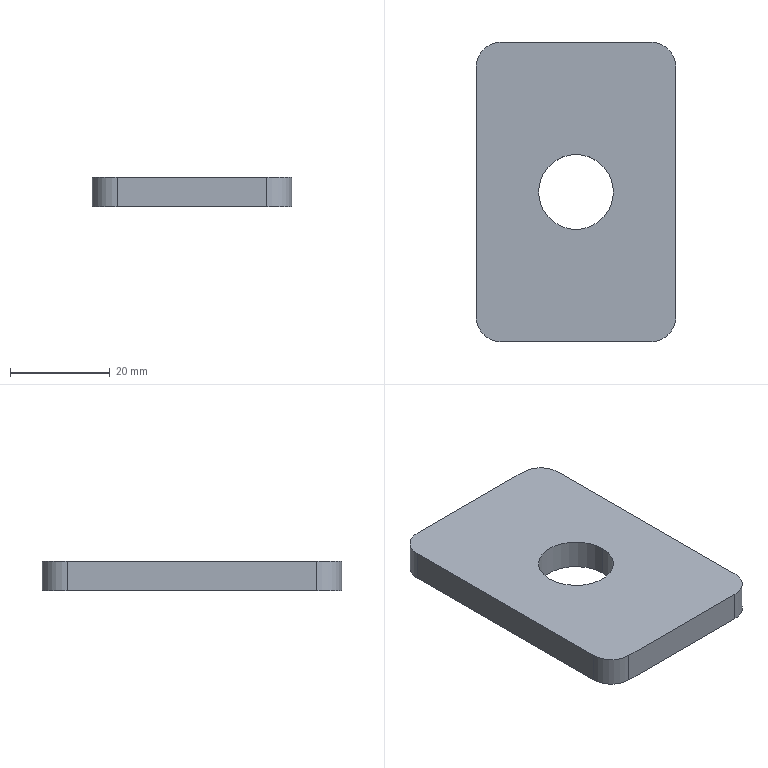Part | SolidWorks | features BaseBody 1 | 1 solid | 12 faces | box 40 x 60 x 6 mm | volume 13211 mm3 | cylinder 6 | plane 6 | commonest cylinder face diameters 10 x4 15 x2
STEP:
#1=CARTESIAN_POINT('',(15.,-30.,6.));
#2=VERTEX_POINT('',#1);
#3=CARTESIAN_POINT('',(20.,-25.,6.));
#4=VERTEX_POINT('',#3);
#5=CARTESIAN_POINT('',(15.,-25.,6.));
#6=DIRECTION('',(0.,0.,1.));
#7=DIRECTION('',(-1.,0.,0.));
#8=AXIS2_PLACEMENT_3D('',#5,#6,#7);
#9=CIRCLE('',#8,5.);
#10=EDGE_CURVE('',#2,#4,#9,.T.);
#11=ORIENTED_EDGE('',*,*,#10,.F.);
#12=CARTESIAN_POINT('',(15.,-30.,0.));
#13=VERTEX_POINT('',#12);
#14=CARTESIAN_POINT('',(15.,-30.,6.));
#15=DIRECTION('',(0.,0.,1.));
#16=VECTOR('',#15,1000.);
#17=LINE('',#14,#16);
#18=EDGE_CURVE('',#13,#2,#17,.T.);
#19=ORIENTED_EDGE('',*,*,#18,.F.);
#20=CARTESIAN_POINT('',(20.,-25.,0.));
#21=VERTEX_POINT('',#20);
#22=CARTESIAN_POINT('',(15.,-25.,0.));
#23=DIRECTION('',(0.,0.,-1.));
#24=DIRECTION('',(-1.,0.,0.));
#25=AXIS2_PLACEMENT_3D('',#22,#23,#24);
#26=CIRCLE('',#25,5.);
#27=EDGE_CURVE('',#21,#13,#26,.T.);
#28=ORIENTED_EDGE('',*,*,#27,.F.);
#29=CARTESIAN_POINT('',(20.,-25.,6.));
#30=DIRECTION('',(0.,0.,-1.));
#31=VECTOR('',#30,1000.);
#32=LINE('',#29,#31);
#33=EDGE_CURVE('',#4,#21,#32,.T.);
#34=ORIENTED_EDGE('',*,*,#33,.F.);
#35=EDGE_LOOP('',(#11,#19,#28,#34));
#36=FACE_OUTER_BOUND('',#35,.T.);
#37=CARTESIAN_POINT('',(15.,-25.,6.));
#38=DIRECTION('',(0.,0.,-1.));
#39=DIRECTION('',(-1.,0.,0.));
#40=AXIS2_PLACEMENT_3D('',#37,#38,#39);
#41=CYLINDRICAL_SURFACE('',#40,5.);
#42=ADVANCED_FACE('',(#36),#41,.T.);
#43=CARTESIAN_POINT('',(-20.,-25.,6.));
#44=VERTEX_POINT('',#43);
#45=CARTESIAN_POINT('',(-15.,-30.,6.));
#46=VERTEX_POINT('',#45);
#47=CARTESIAN_POINT('',(-15.,-25.,6.));
#48=DIRECTION('',(0.,0.,1.));
#49=DIRECTION('',(-1.,0.,0.));
#50=AXIS2_PLACEMENT_3D('',#47,#48,#49);
#51=CIRCLE('',#50,5.);
#52=EDGE_CURVE('',#44,#46,#51,.T.);
#53=ORIENTED_EDGE('',*,*,#52,.F.);
#54=CARTESIAN_POINT('',(-20.,-25.,0.));
#55=VERTEX_POINT('',#54);
#56=CARTESIAN_POINT('',(-20.,-25.,6.));
#57=DIRECTION('',(0.,0.,1.));
#58=VECTOR('',#57,1000.);
#59=LINE('',#56,#58);
#60=EDGE_CURVE('',#55,#44,#59,.T.);
#61=ORIENTED_EDGE('',*,*,#60,.F.);
#62=CARTESIAN_POINT('',(-15.,-30.,0.));
#63=VERTEX_POINT('',#62);
#64=CARTESIAN_POINT('',(-15.,-25.,0.));
#65=DIRECTION('',(0.,0.,-1.));
#66=DIRECTION('',(-1.,0.,0.));
#67=AXIS2_PLACEMENT_3D('',#64,#65,#66);
#68=CIRCLE('',#67,5.);
#69=EDGE_CURVE('',#63,#55,#68,.T.);
#70=ORIENTED_EDGE('',*,*,#69,.F.);
#71=CARTESIAN_POINT('',(-15.,-30.,6.));
#72=DIRECTION('',(0.,0.,-1.));
#73=VECTOR('',#72,1000.);
#74=LINE('',#71,#73);
#75=EDGE_CURVE('',#46,#63,#74,.T.);
#76=ORIENTED_EDGE('',*,*,#75,.F.);
#77=EDGE_LOOP('',(#53,#61,#70,#76));
#78=FACE_OUTER_BOUND('',#77,.T.);
#79=CARTESIAN_POINT('',(-15.,-25.,6.));
#80=DIRECTION('',(0.,0.,-1.));
#81=DIRECTION('',(-1.,0.,0.));
#82=AXIS2_PLACEMENT_3D('',#79,#80,#81);
#83=CYLINDRICAL_SURFACE('',#82,5.);
#84=ADVANCED_FACE('',(#78),#83,.T.);
#85=CARTESIAN_POINT('',(-15.,30.,6.));
#86=VERTEX_POINT('',#85);
#87=CARTESIAN_POINT('',(-20.,25.,6.));
#88=VERTEX_POINT('',#87);
#89=CARTESIAN_POINT('',(-15.,25.,6.));
#90=DIRECTION('',(0.,0.,1.));
#91=DIRECTION('',(-1.,0.,0.));
#92=AXIS2_PLACEMENT_3D('',#89,#90,#91);
#93=CIRCLE('',#92,5.);
#94=EDGE_CURVE('',#86,#88,#93,.T.);
#95=ORIENTED_EDGE('',*,*,#94,.F.);
#96=CARTESIAN_POINT('',(-15.,30.,0.));
#97=VERTEX_POINT('',#96);
#98=CARTESIAN_POINT('',(-15.,30.,6.));
#99=DIRECTION('',(0.,0.,1.));
#100=VECTOR('',#99,1000.);
#101=LINE('',#98,#100);
#102=EDGE_CURVE('',#97,#86,#101,.T.);
#103=ORIENTED_EDGE('',*,*,#102,.F.);
#104=CARTESIAN_POINT('',(-20.,25.,0.));
#105=VERTEX_POINT('',#104);
#106=CARTESIAN_POINT('',(-15.,25.,0.));
#107=DIRECTION('',(0.,0.,-1.));
#108=DIRECTION('',(-1.,0.,0.));
#109=AXIS2_PLACEMENT_3D('',#106,#107,#108);
#110=CIRCLE('',#109,5.);
#111=EDGE_CURVE('',#105,#97,#110,.T.);
#112=ORIENTED_EDGE('',*,*,#111,.F.);
#113=CARTESIAN_POINT('',(-20.,25.,6.));
#114=DIRECTION('',(0.,0.,-1.));
#115=VECTOR('',#114,1000.);
#116=LINE('',#113,#115);
#117=EDGE_CURVE('',#88,#105,#116,.T.);
#118=ORIENTED_EDGE('',*,*,#117,.F.);
#119=EDGE_LOOP('',(#95,#103,#112,#118));
#120=FACE_OUTER_BOUND('',#119,.T.);
#121=CARTESIAN_POINT('',(-15.,25.,6.));
#122=DIRECTION('',(0.,0.,-1.));
#123=DIRECTION('',(-1.,0.,0.));
#124=AXIS2_PLACEMENT_3D('',#121,#122,#123);
#125=CYLINDRICAL_SURFACE('',#124,5.);
#126=ADVANCED_FACE('',(#120),#125,.T.);
#127=CARTESIAN_POINT('',(20.,25.,6.));
#128=VERTEX_POINT('',#127);
#129=CARTESIAN_POINT('',(15.,30.,6.));
#130=VERTEX_POINT('',#129);
#131=CARTESIAN_POINT('',(15.,25.,6.));
#132=DIRECTION('',(0.,0.,1.));
#133=DIRECTION('',(-1.,0.,0.));
#134=AXIS2_PLACEMENT_3D('',#131,#132,#133);
#135=CIRCLE('',#134,5.);
#136=EDGE_CURVE('',#128,#130,#135,.T.);
#137=ORIENTED_EDGE('',*,*,#136,.F.);
#138=CARTESIAN_POINT('',(20.,25.,0.));
#139=VERTEX_POINT('',#138);
#140=CARTESIAN_POINT('',(20.,25.,6.));
#141=DIRECTION('',(0.,0.,1.));
#142=VECTOR('',#141,1000.);
#143=LINE('',#140,#142);
#144=EDGE_CURVE('',#139,#128,#143,.T.);
#145=ORIENTED_EDGE('',*,*,#144,.F.);
#146=CARTESIAN_POINT('',(15.,30.,0.));
#147=VERTEX_POINT('',#146);
#148=CARTESIAN_POINT('',(15.,25.,0.));
#149=DIRECTION('',(0.,0.,-1.));
#150=DIRECTION('',(-1.,0.,0.));
#151=AXIS2_PLACEMENT_3D('',#148,#149,#150);
#152=CIRCLE('',#151,5.);
#153=EDGE_CURVE('',#147,#139,#152,.T.);
#154=ORIENTED_EDGE('',*,*,#153,.F.);
#155=CARTESIAN_POINT('',(15.,30.,6.));
#156=DIRECTION('',(0.,0.,-1.));
#157=VECTOR('',#156,1000.);
#158=LINE('',#155,#157);
#159=EDGE_CURVE('',#130,#147,#158,.T.);
#160=ORIENTED_EDGE('',*,*,#159,.F.);
#161=EDGE_LOOP('',(#137,#145,#154,#160));
#162=FACE_OUTER_BOUND('',#161,.T.);
#163=CARTESIAN_POINT('',(15.,25.,6.));
#164=DIRECTION('',(0.,0.,-1.));
#165=DIRECTION('',(-1.,0.,0.));
#166=AXIS2_PLACEMENT_3D('',#163,#164,#165);
#167=CYLINDRICAL_SURFACE('',#166,5.);
#168=ADVANCED_FACE('',(#162),#167,.T.);
#169=CARTESIAN_POINT('',(-7.5,0.,0.));
#170=VERTEX_POINT('',#169);
#171=CARTESIAN_POINT('',(-7.5,0.,6.));
#172=VERTEX_POINT('',#171);
#173=CARTESIAN_POINT('',(-7.5,0.,0.));
#174=DIRECTION('',(0.,0.,1.));
#175=VECTOR('',#174,1000.);
#176=LINE('',#173,#175);
#177=EDGE_CURVE('',#170,#172,#176,.T.);
#178=ORIENTED_EDGE('',*,*,#177,.F.);
#179=CARTESIAN_POINT('',(7.5,0.,0.));
#180=VERTEX_POINT('',#179);
#181=CARTESIAN_POINT('',(0.,0.,0.));
#182=DIRECTION('',(0.,0.,1.));
#183=DIRECTION('',(1.,0.,0.));
#184=AXIS2_PLACEMENT_3D('',#181,#182,#183);
#185=CIRCLE('',#184,7.5);
#186=EDGE_CURVE('',#180,#170,#185,.T.);
#187=ORIENTED_EDGE('',*,*,#186,.F.);
#188=CARTESIAN_POINT('',(7.5,0.,6.));
#189=VERTEX_POINT('',#188);
#190=CARTESIAN_POINT('',(7.5,0.,0.));
#191=DIRECTION('',(0.,0.,1.));
#192=VECTOR('',#191,1000.);
#193=LINE('',#190,#192);
#194=EDGE_CURVE('',#180,#189,#193,.T.);
#195=ORIENTED_EDGE('',*,*,#194,.T.);
#196=CARTESIAN_POINT('',(0.,0.,6.));
#197=DIRECTION('',(0.,0.,1.));
#198=DIRECTION('',(1.,0.,0.));
#199=AXIS2_PLACEMENT_3D('',#196,#197,#198);
#200=CIRCLE('',#199,7.5);
#201=EDGE_CURVE('',#189,#172,#200,.T.);
#202=ORIENTED_EDGE('',*,*,#201,.T.);
#203=EDGE_LOOP('',(#178,#187,#195,#202));
#204=FACE_OUTER_BOUND('',#203,.T.);
#205=CARTESIAN_POINT('',(0.,0.,0.));
#206=DIRECTION('',(0.,0.,1.));
#207=DIRECTION('',(1.,0.,0.));
#208=AXIS2_PLACEMENT_3D('',#205,#206,#207);
#209=CYLINDRICAL_SURFACE('',#208,7.5);
#210=ADVANCED_FACE('',(#204),#209,.F.);
#211=ORIENTED_EDGE('',*,*,#186,.T.);
#212=CARTESIAN_POINT('',(0.,0.,0.));
#213=DIRECTION('',(0.,0.,1.));
#214=DIRECTION('',(1.,0.,0.));
#215=AXIS2_PLACEMENT_3D('',#212,#213,#214);
#216=CIRCLE('',#215,7.5);
#217=EDGE_CURVE('',#170,#180,#216,.T.);
#218=ORIENTED_EDGE('',*,*,#217,.T.);
#219=EDGE_LOOP('',(#211,#218));
#220=FACE_BOUND('',#219,.T.);
#221=CARTESIAN_POINT('',(-20.,30.,0.));
#222=DIRECTION('',(-1.,0.,0.));
#223=VECTOR('',#222,1000.);
#224=LINE('',#221,#223);
#225=EDGE_CURVE('',#147,#97,#224,.T.);
#226=ORIENTED_EDGE('',*,*,#225,.F.);
#227=ORIENTED_EDGE('',*,*,#153,.T.);
#228=CARTESIAN_POINT('',(20.,-30.,0.));
#229=DIRECTION('',(0.,1.,0.));
#230=VECTOR('',#229,1000.);
#231=LINE('',#228,#230);
#232=EDGE_CURVE('',#21,#139,#231,.T.);
#233=ORIENTED_EDGE('',*,*,#232,.F.);
#234=ORIENTED_EDGE('',*,*,#27,.T.);
#235=CARTESIAN_POINT('',(-20.,-30.,0.));
#236=DIRECTION('',(1.,0.,0.));
#237=VECTOR('',#236,1000.);
#238=LINE('',#235,#237);
#239=EDGE_CURVE('',#63,#13,#238,.T.);
#240=ORIENTED_EDGE('',*,*,#239,.F.);
#241=ORIENTED_EDGE('',*,*,#69,.T.);
#242=CARTESIAN_POINT('',(-20.,-30.,0.));
#243=DIRECTION('',(0.,-1.,0.));
#244=VECTOR('',#243,1000.);
#245=LINE('',#242,#244);
#246=EDGE_CURVE('',#105,#55,#245,.T.);
#247=ORIENTED_EDGE('',*,*,#246,.F.);
#248=ORIENTED_EDGE('',*,*,#111,.T.);
#249=EDGE_LOOP('',(#226,#227,#233,#234,#240,#241,#247,#248));
#250=FACE_OUTER_BOUND('',#249,.T.);
#251=CARTESIAN_POINT('',(0.,0.,0.));
#252=DIRECTION('',(0.,0.,-1.));
#253=DIRECTION('',(0.,-1.,0.));
#254=AXIS2_PLACEMENT_3D('',#251,#252,#253);
#255=PLANE('',#254);
#256=ADVANCED_FACE('',(#220,#250),#255,.T.);
#257=ORIENTED_EDGE('',*,*,#201,.F.);
#258=CARTESIAN_POINT('',(0.,0.,6.));
#259=DIRECTION('',(0.,0.,1.));
#260=DIRECTION('',(1.,0.,0.));
#261=AXIS2_PLACEMENT_3D('',#258,#259,#260);
#262=CIRCLE('',#261,7.5);
#263=EDGE_CURVE('',#172,#189,#262,.T.);
#264=ORIENTED_EDGE('',*,*,#263,.F.);
#265=EDGE_LOOP('',(#257,#264));
#266=FACE_BOUND('',#265,.T.);
#267=CARTESIAN_POINT('',(20.,-30.,6.));
#268=DIRECTION('',(0.,1.,0.));
#269=VECTOR('',#268,1000.);
#270=LINE('',#267,#269);
#271=EDGE_CURVE('',#4,#128,#270,.T.);
#272=ORIENTED_EDGE('',*,*,#271,.T.);
#273=ORIENTED_EDGE('',*,*,#136,.T.);
#274=CARTESIAN_POINT('',(-20.,30.,6.));
#275=DIRECTION('',(-1.,0.,0.));
#276=VECTOR('',#275,1000.);
#277=LINE('',#274,#276);
#278=EDGE_CURVE('',#130,#86,#277,.T.);
#279=ORIENTED_EDGE('',*,*,#278,.T.);
#280=ORIENTED_EDGE('',*,*,#94,.T.);
#281=CARTESIAN_POINT('',(-20.,-30.,6.));
#282=DIRECTION('',(0.,-1.,0.));
#283=VECTOR('',#282,1000.);
#284=LINE('',#281,#283);
#285=EDGE_CURVE('',#88,#44,#284,.T.);
#286=ORIENTED_EDGE('',*,*,#285,.T.);
#287=ORIENTED_EDGE('',*,*,#52,.T.);
#288=CARTESIAN_POINT('',(-20.,-30.,6.));
#289=DIRECTION('',(1.,0.,0.));
#290=VECTOR('',#289,1000.);
#291=LINE('',#288,#290);
#292=EDGE_CURVE('',#46,#2,#291,.T.);
#293=ORIENTED_EDGE('',*,*,#292,.T.);
#294=ORIENTED_EDGE('',*,*,#10,.T.);
#295=EDGE_LOOP('',(#272,#273,#279,#280,#286,#287,#293,#294));
#296=FACE_OUTER_BOUND('',#295,.T.);
#297=CARTESIAN_POINT('',(0.,0.,6.));
#298=DIRECTION('',(0.,0.,-1.));
#299=DIRECTION('',(0.,-1.,0.));
#300=AXIS2_PLACEMENT_3D('',#297,#298,#299);
#301=PLANE('',#300);
#302=ADVANCED_FACE('',(#266,#296),#301,.F.);
#303=ORIENTED_EDGE('',*,*,#292,.F.);
#304=ORIENTED_EDGE('',*,*,#75,.T.);
#305=ORIENTED_EDGE('',*,*,#239,.T.);
#306=ORIENTED_EDGE('',*,*,#18,.T.);
#307=EDGE_LOOP('',(#303,#304,#305,#306));
#308=FACE_OUTER_BOUND('',#307,.T.);
#309=CARTESIAN_POINT('',(-20.,-30.,6.));
#310=DIRECTION('',(0.,1.,0.));
#311=DIRECTION('',(1.,0.,0.));
#312=AXIS2_PLACEMENT_3D('',#309,#310,#311);
#313=PLANE('',#312);
#314=ADVANCED_FACE('',(#308),#313,.F.);
#315=ORIENTED_EDGE('',*,*,#285,.F.);
#316=ORIENTED_EDGE('',*,*,#117,.T.);
#317=ORIENTED_EDGE('',*,*,#246,.T.);
#318=ORIENTED_EDGE('',*,*,#60,.T.);
#319=EDGE_LOOP('',(#315,#316,#317,#318));
#320=FACE_OUTER_BOUND('',#319,.T.);
#321=CARTESIAN_POINT('',(-20.,-30.,6.));
#322=DIRECTION('',(1.,0.,0.));
#323=DIRECTION('',(0.,1.,0.));
#324=AXIS2_PLACEMENT_3D('',#321,#322,#323);
#325=PLANE('',#324);
#326=ADVANCED_FACE('',(#320),#325,.F.);
#327=ORIENTED_EDGE('',*,*,#278,.F.);
#328=ORIENTED_EDGE('',*,*,#159,.T.);
#329=ORIENTED_EDGE('',*,*,#225,.T.);
#330=ORIENTED_EDGE('',*,*,#102,.T.);
#331=EDGE_LOOP('',(#327,#328,#329,#330));
#332=FACE_OUTER_BOUND('',#331,.T.);
#333=CARTESIAN_POINT('',(-20.,30.,6.));
#334=DIRECTION('',(0.,-1.,0.));
#335=DIRECTION('',(0.,0.,-1.));
#336=AXIS2_PLACEMENT_3D('',#333,#334,#335);
#337=PLANE('',#336);
#338=ADVANCED_FACE('',(#332),#337,.F.);
#339=ORIENTED_EDGE('',*,*,#232,.T.);
#340=ORIENTED_EDGE('',*,*,#144,.T.);
#341=ORIENTED_EDGE('',*,*,#271,.F.);
#342=ORIENTED_EDGE('',*,*,#33,.T.);
#343=EDGE_LOOP('',(#339,#340,#341,#342));
#344=FACE_OUTER_BOUND('',#343,.T.);
#345=CARTESIAN_POINT('',(20.,-30.,6.));
#346=DIRECTION('',(-1.,0.,0.));
#347=DIRECTION('',(0.,0.,1.));
#348=AXIS2_PLACEMENT_3D('',#345,#346,#347);
#349=PLANE('',#348);
#350=ADVANCED_FACE('',(#344),#349,.F.);
#351=ORIENTED_EDGE('',*,*,#217,.F.);
#352=ORIENTED_EDGE('',*,*,#177,.T.);
#353=ORIENTED_EDGE('',*,*,#263,.T.);
#354=ORIENTED_EDGE('',*,*,#194,.F.);
#355=EDGE_LOOP('',(#351,#352,#353,#354));
#356=FACE_OUTER_BOUND('',#355,.T.);
#357=CARTESIAN_POINT('',(0.,0.,0.));
#358=DIRECTION('',(0.,0.,1.));
#359=DIRECTION('',(1.,0.,0.));
#360=AXIS2_PLACEMENT_3D('',#357,#358,#359);
#361=CYLINDRICAL_SURFACE('',#360,7.5);
#362=ADVANCED_FACE('',(#356),#361,.F.);
#363=CLOSED_SHELL('',(#42,#84,#126,#168,#210,#256,#302,#314,#326,#338,#350,#362));
#364=MANIFOLD_SOLID_BREP('',#363);
#365=CARTESIAN_POINT('',(0.,0.,0.));
#366=DIRECTION('',(0.,0.,1.));
#367=DIRECTION('',(1.,0.,0.));
#368=AXIS2_PLACEMENT_3D('',#365,#366,#367);
#369=(LENGTH_UNIT()NAMED_UNIT(*)SI_UNIT(.MILLI.,.METRE.));
#370=UNCERTAINTY_MEASURE_WITH_UNIT(LENGTH_MEASURE(0.00001),#369,'','');
#371=(NAMED_UNIT(*)PLANE_ANGLE_UNIT()SI_UNIT($,.RADIAN.));
#372=(NAMED_UNIT(*)SI_UNIT($,.STERADIAN.)SOLID_ANGLE_UNIT());
#373=(GEOMETRIC_REPRESENTATION_CONTEXT(3)GLOBAL_UNCERTAINTY_ASSIGNED_CONTEXT((#370))GLOBAL_UNIT_ASSIGNED_CONTEXT((#369,#371,#372))REPRESENTATION_CONTEXT('',''));
#374=ADVANCED_BREP_SHAPE_REPRESENTATION('',(#364,#368),#373);